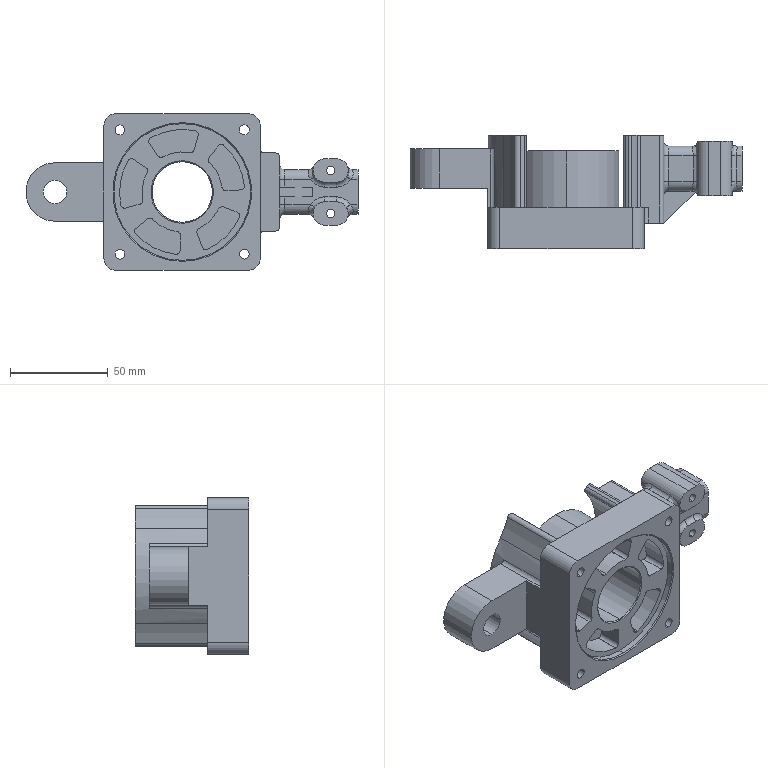Part | STEP file | Belt polisher base | 1 solid | 225 faces | box 170 x 58 x 80 mm | volume 200572 mm3 | cylinder 128 | plane 59 | cone 16 | torus 12 | spline 10 | commonest cylinder face diameters 4 x39 5 x27 12 x12 3.3 x8 10 x8 41 x5